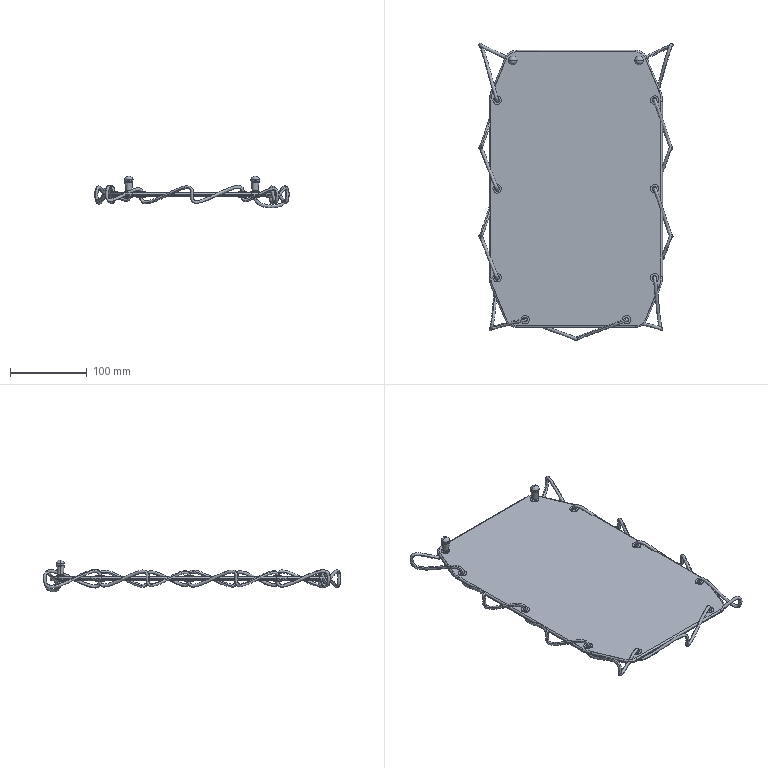Part | SolidWorks | 6 solids | 277 faces | box 252.714 x 386.443 x 41.666 mm | volume 416549 mm3 | cylinder 195 | plane 40 | torus 20 | cone 12 | sphere 8 | spline 2 | commonest cylinder face diameters 11.001 x80 6 x59 4 x36 31.931 x8 7.8 x4 9.2 x4